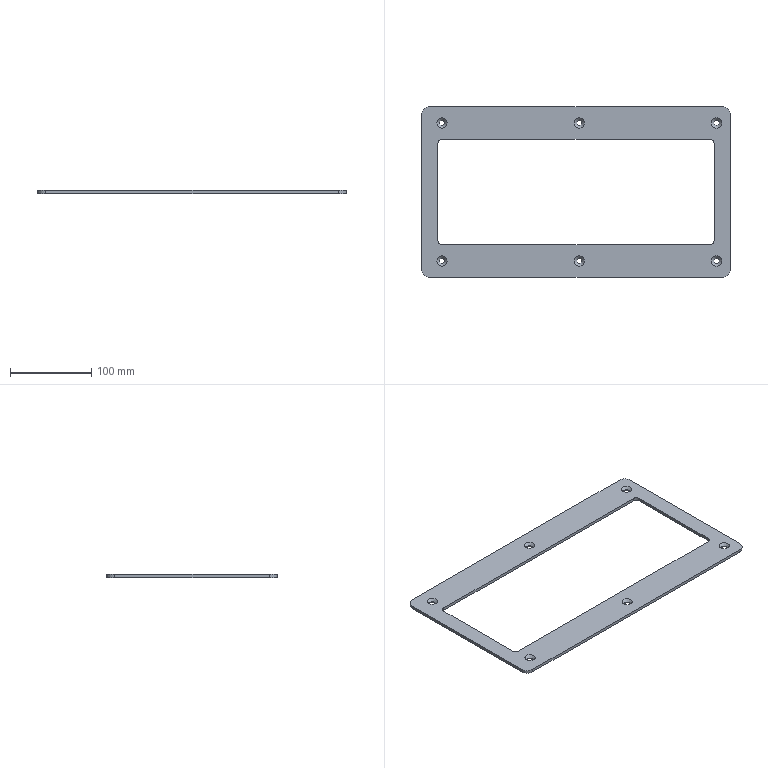CAM job | NX | 3-axis milling | part box 380 x 210 x 3.7 mm | stock box 386 x 216 x 4.7 mm
Operations:
program,operation,operation_type,tool,method,geometry_group,spindle_rpm,surface_speed,feed_per_tooth,feed_cut,feed_plunge,cut_length_mm,path_length_mm,cut_time_min,machine_time_min
385-215-4毛胚-吸盘,FLOOR_WALL,VolumeBased25DMillingOperation,D10,METHOD,A,6500.0,0.0,0.0,1250.0,100.0,11311.997,11365.997,9.05,9.055
385-215-4毛胚-吸盘,ZLEVEL_PROFILE,ZLevelMilling,D10,METHOD,A,6500.0,326.0,0.1538,2000.0,1000.0,8566.546,8737.694,4.328,4.345
385-215-4毛胚-吸盘,ZLEVEL_PROFILE_COPY_COPY_1_COPY_COPY_1_COPY,ZLevelMilling,D4,METHOD,A,7000.0,87.0,0.1429,2000.0,1000.0,9655.247,10881.586,4.916,5.038
385-215-4毛胚-吸盘,ZLEVEL_PROFILE_COPY_1_COPY_COPY_COPY_COPY_COPY_COPY,ZLevelMilling,D6A45,METHOD,A,7000.0,131.0,0.0714,1000.0,1000.0,2101.17,2572.978,2.101,2.148
385-215-4毛胚-吸盘,ZLEVEL_PROFILE_COPY_COPY_1_COPY,ZLevelMilling,D4,METHOD,A,6000.0,75.0,0.0833,1000.0,1000.0,2105.424,2581.617,2.105,2.153